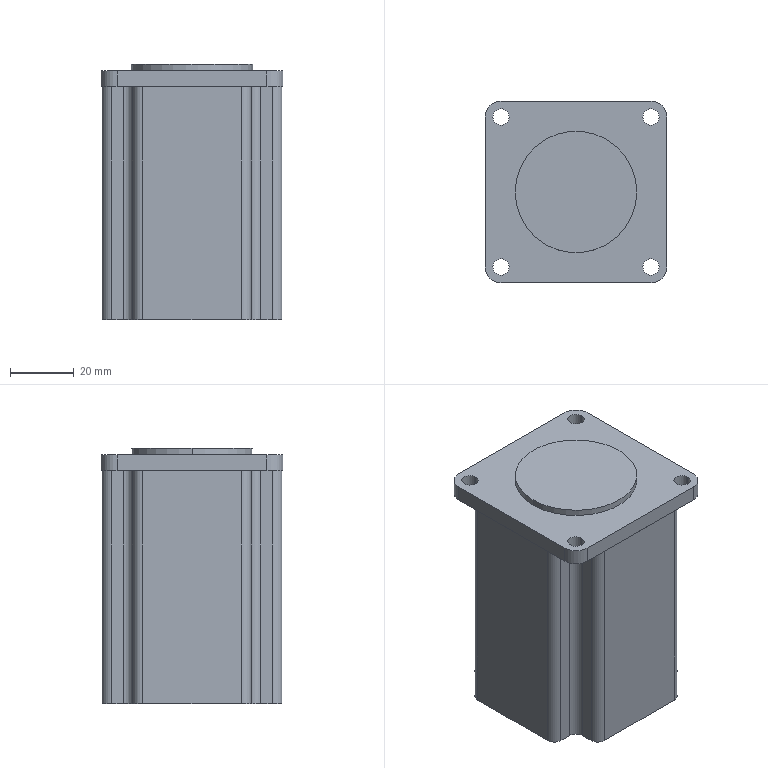Part | STEP file | 57 stepper motor 001 | 3 solids | 48 faces | box 57 x 57 x 80 mm | volume 221641 mm3 | cylinder 26 | plane 22 | commonest cylinder face diameters 6 x12 5.1 x8 10 x4 38.1 x2